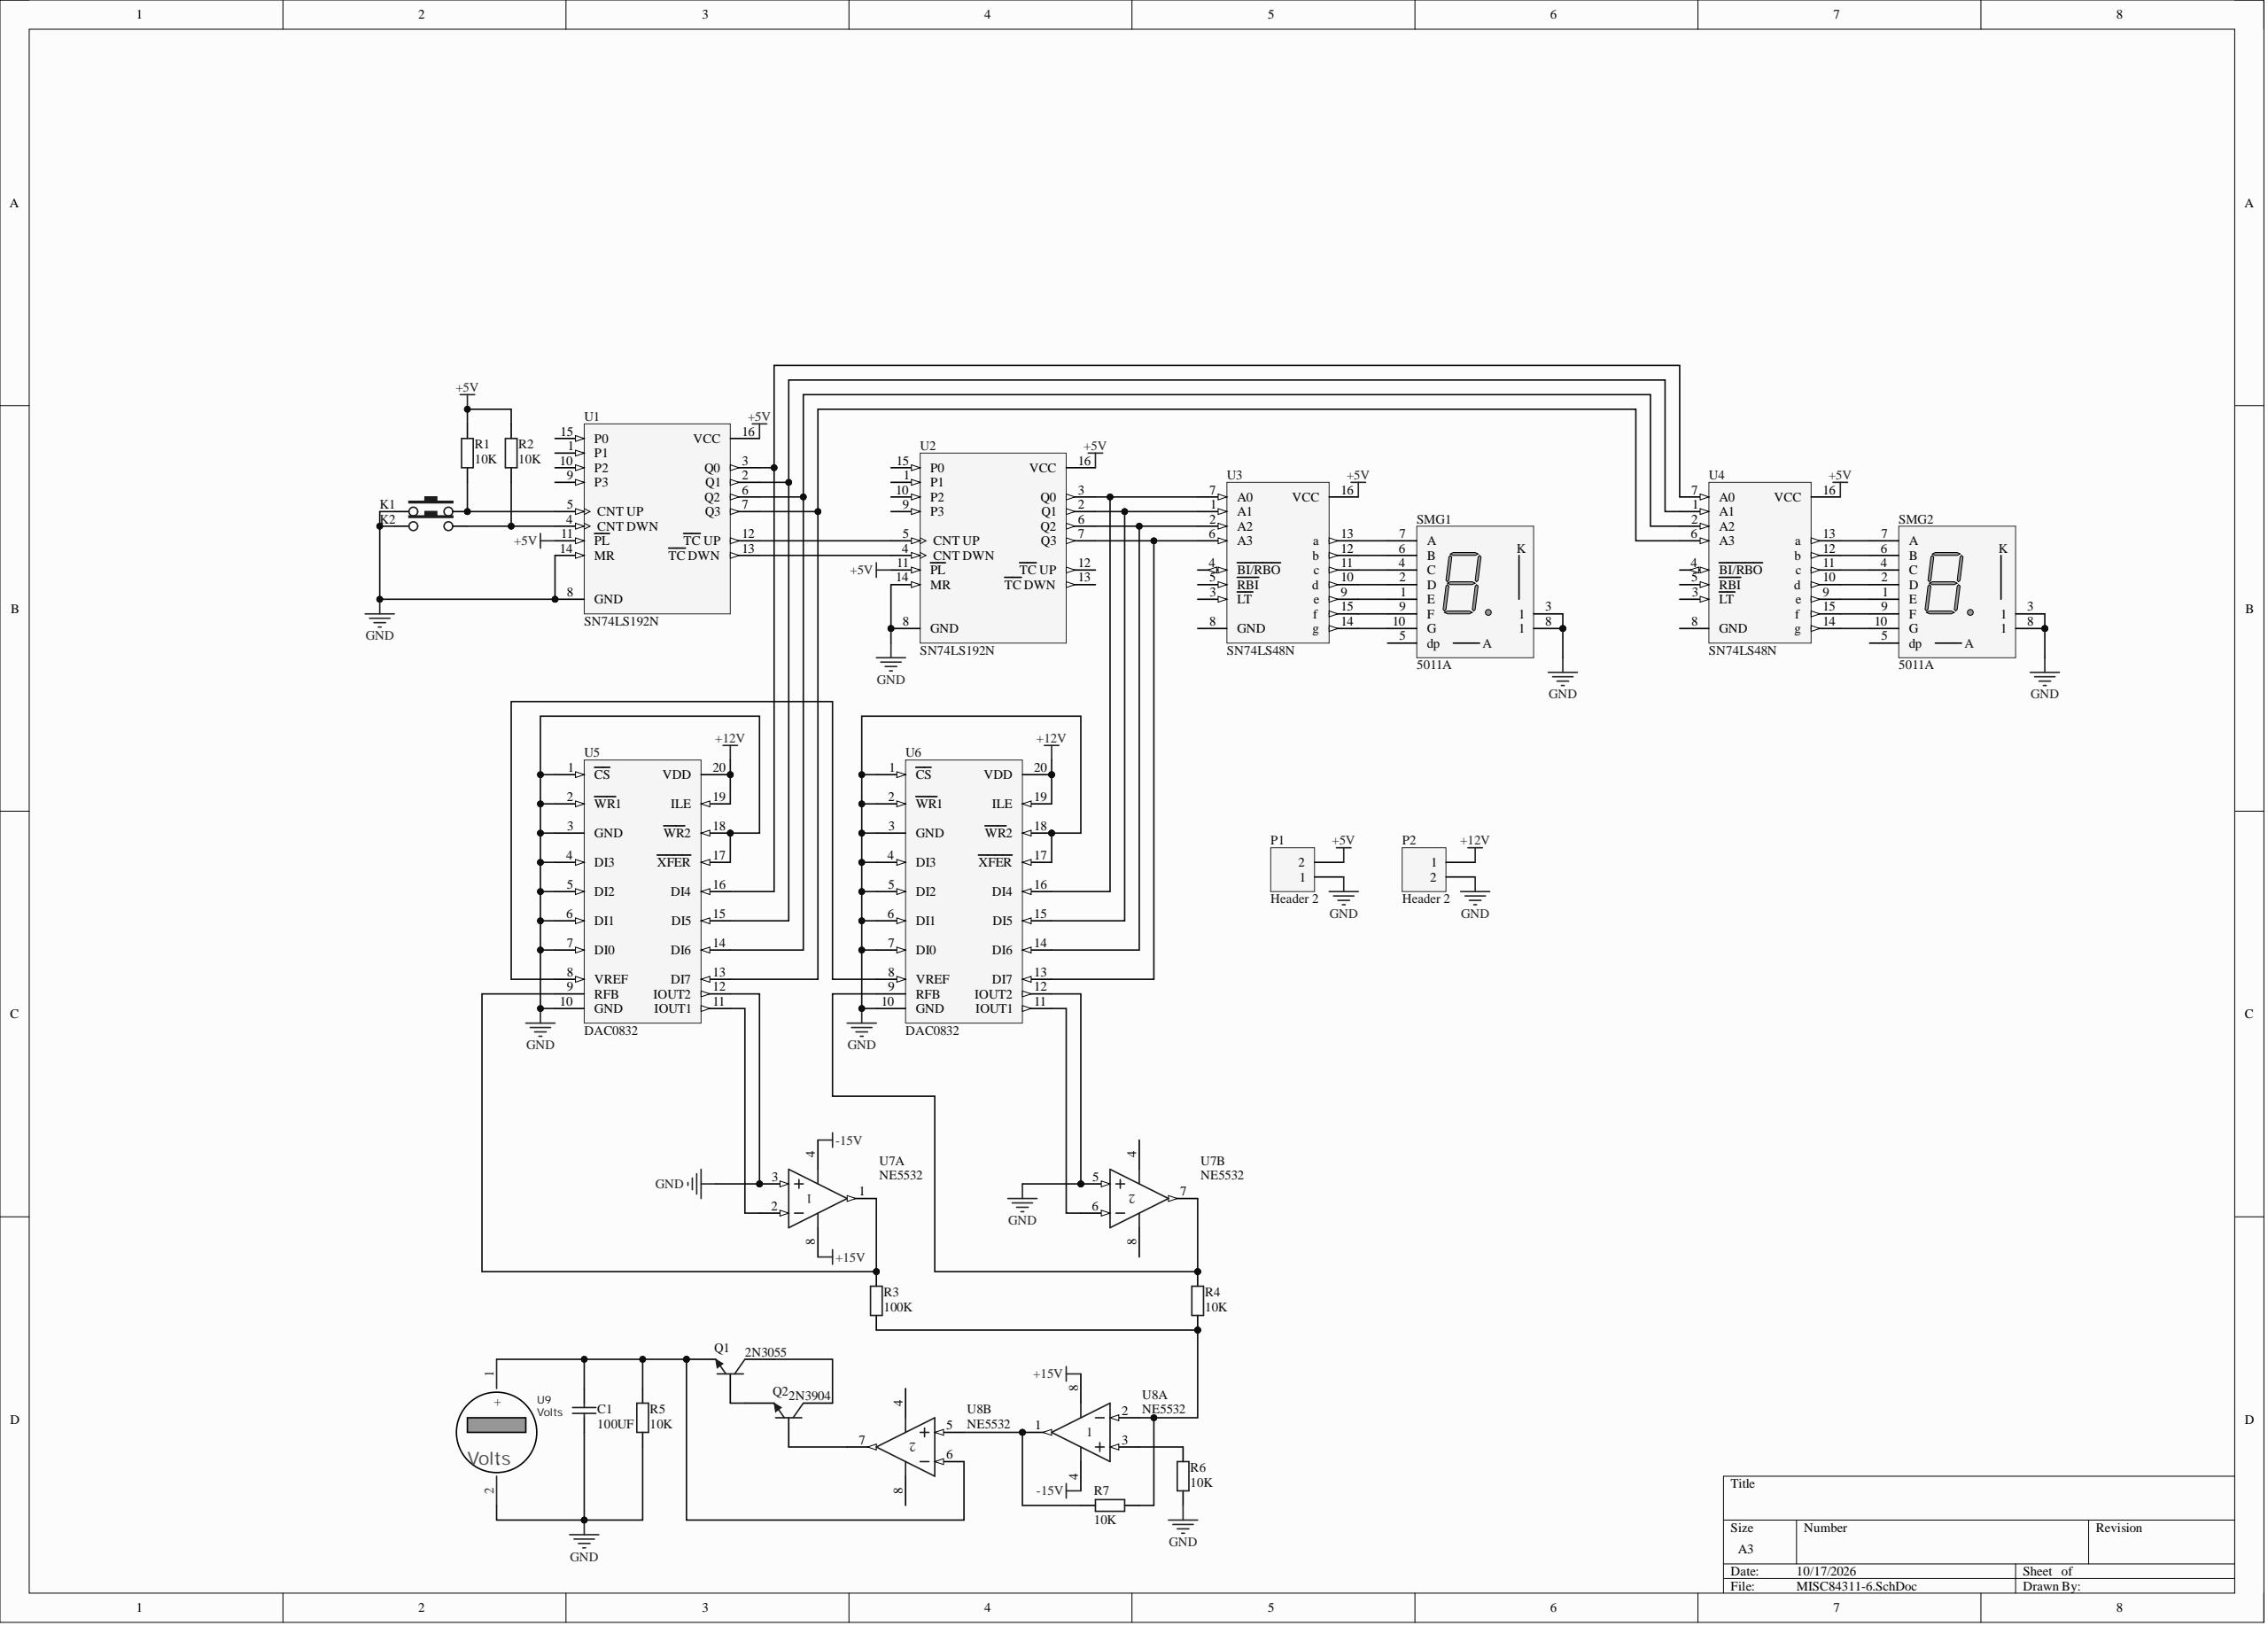Circuit board | Altium Designer | 25 parts | 43 nets
Bill of materials:
Comment,Description,Designator,Footprint,LibRef,Quantity
"100UF","Capacitor","C1","RAD-0.3","Cap","1"
"KEY","","K1, K2","DIP-3X6X4.3","KEY","2"
"Header 2","Header, 2-Pin","P1, P2","HDR1X2","Header 2","2"
"2N3055","NPN General Purpose Amplifier","Q1","TO-92A","2N3904","1"
"2N3904","NPN General Purpose Amplifier","Q2","TO-92A","2N3904","1"
"10K","Color-band resistor","R1, R2, R4, R5, R6, R7","RS 1/4W","R-S","6"
"100K","Color-band resistor","R3","RS 1/4W","R-S","1"
"5011A","0.5-inch 1-digit common-cathode seven-segment display","SMG1, SMG2","SMG 0.5-1P","5011A","2"
"SN74LS192N","Presettable BCD Decade Up/Down Counter","U1, U2","648-08","SN74LS192N","2"
"SN74LS48N","BCD-to-Seven-Segment Decoder/Driver","U3, U4","N016D","SN74LS48N","2"
"DAC0832","8-Bit uP-Compatible, Double-Buffered Digital-to-Analog Converter","U5, U6","J20A","DAC0832LCJ","2"
"NE5532","Dual Low-Noise Operational Amplifier","U7, U8","P008","NE5532AP","2"
"Volts","","U9","CAPACITANCE 1 FARAD 5,5 VOLT","Volts","1"
Netlist (Protel format):
[
C1
RAD-0.3
100UF



]
[
K1
DIP-3X6X4.3
KEY



]
[
K2
DIP-3X6X4.3
KEY



]
[
P1
HDR1X2
Header 2



]
[
P2
HDR1X2
Header 2



]
[
Q1
TO-92A
2N3055



]
[
Q2
TO-92A
2N3904



]
[
R1
RS 1/4W
10K



]
[
R2
RS 1/4W
10K



]
[
R3
RS 1/4W
100K



]
[
R4
RS 1/4W
10K



]
[
R5
RS 1/4W
10K



]
[
R6
RS 1/4W
10K



]
[
R7
RS 1/4W
10K



]
[
SMG1
SMG 0.5-1P
5011A



]
[
SMG2
SMG 0.5-1P
5011A



]
[
U1
648-08
SN74LS192N



]
[
U2
648-08
SN74LS192N



]
[
U3
N016D
SN74LS48N



]
[
U4
N016D
SN74LS48N



]
[
U5
J20A
DAC0832



]
[
U6
J20A
DAC0832



]
[
U7
P008
NE5532



]
[
U8
P008
NE5532



]
[
U9
CAPACITANCE 1 FARAD 5,5 VOLT
Volts



]
(
NetU6_11
U6-11
U7-6
)
(
NetU5_11
U5-11
U7-2
)
(
NetU5_8
U5-8
U6-8
)
(
NetU2_7
U2-7
U3-6
U6-13
)
(
NetU2_6
U2-6
U3-2
U6-14
)
(
NetU2_3
U2-3
U3-7
U6-16
)
(
NetU2_2
U2-2
U3-1
U6-15
)
(
NetU1_13
U1-13
U2-4
)
(
NetU1_12
U1-12
U2-5
)
(
NetU1_7
U1-7
U4-6
U5-13
)
(
NetU1_6
U1-6
U4-2
U5-14
)
(
NetU1_3
U1-3
U4-7
U5-16
)
(
NetU1_2
U1-2
U4-1
U5-15
)
(
NetSMG2_10
SMG2-10
U4-14
)
(
NetSMG2_9
SMG2-9
U4-15
)
(
NetSMG2_7
SMG2-7
U4-13
)
(
NetSMG2_6
SMG2-6
U4-12
)
(
NetSMG2_4
SMG2-4
U4-11
)
(
NetSMG2_2
SMG2-2
U4-10
)
(
NetSMG2_1
SMG2-1
U4-9
)
(
NetSMG1_10
SMG1-10
U3-14
)
(
NetSMG1_9
SMG1-9
U3-15
)
(
NetSMG1_7
SMG1-7
U3-13
)
(
NetSMG1_6
SMG1-6
U3-12
)
(
NetSMG1_4
SMG1-4
U3-11
)
(
NetSMG1_2
SMG1-2
U3-10
)
(
NetSMG1_1
SMG1-1
U3-9
)
(
NetR7_2
R7-2
U8-1
U8-5
)
(
NetR6_2
R6-2
U8-3
)
(
NetR4_2
R4-2
U6-9
U7-7
)
(
NetR3_2
R3-2
U5-9
U7-1
)
(
NetR3_1
R3-1
R4-1
R7-1
U8-2
)
(
NetQ2_2
Q2-2
U8-7
)
(
NetQ1_3
Q1-3
Q2-3
)
(
NetQ1_2
Q1-2
Q2-1
)
(
NetK2_3
K2-3
R2-1
U1-4
)
(
NetK1_3
K1-3
R1-1
U1-5
)
(
NetC1_2
C1-2
Q1-1
R5-1
U8-6
U9-1
)
(
GND
C1-1
K1-1
K2-1
P1-1
P2-2
R5-2
R6-1
SMG1-3
SMG1-8
SMG2-3
SMG2-8
U1-8
U1-14
U2-8
U2-14
U5-1
U5-2
U5-3
U5-4
U5-5
U5-6
U5-7
U5-10
U5-12
U5-17
U5-18
U6-1
U6-2
U6-3
U6-4
U6-5
U6-6
U6-7
U6-10
U6-12
U6-17
U6-18
U7-3
U7-5
U9-2
)
(
-15V
U7-4
U8-4
)
(
+15V
U7-8
U8-8
)
(
+12V
P2-1
U5-19
U5-20
U6-19
U6-20
)
(
+5V
P1-2
R1-2
R2-2
U1-11
U1-16
U2-11
U2-16
U3-16
U4-16
)